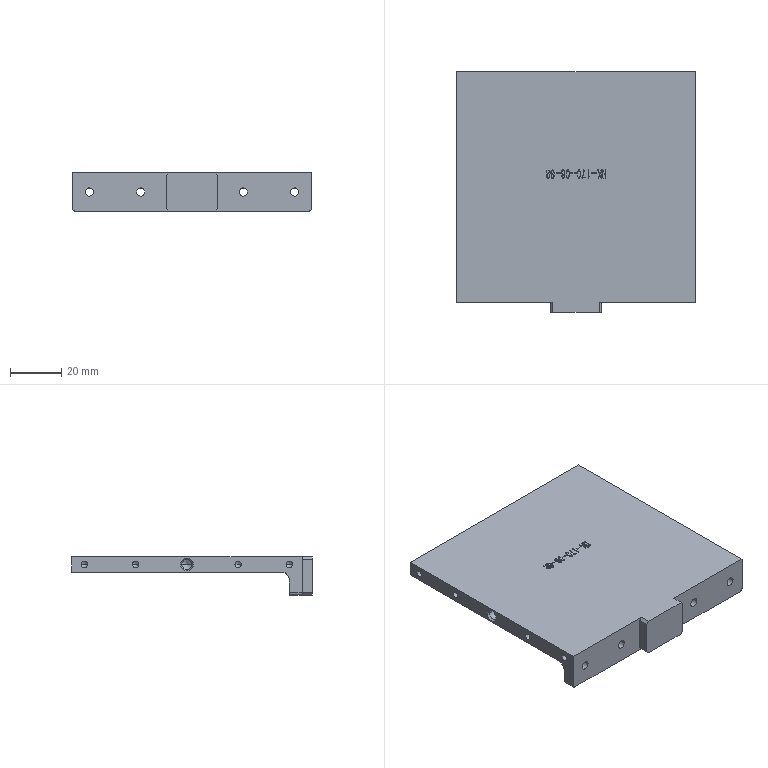NC program | NX | posted with a generic post | part box 93.2 x 94 x 15 mm
Whole program, first 2058 of 2264 lines:
N10 G17 G21 G94 G90
(FLOOR_WALL , TOOL : D10)
N12 T15 M6
N14 G54
N16 G17 G0 G90 X51. Y54.6 B0. C0. S9500 M3
N18 G43 Z30. H15
N20 Z-5.9
N22 G94 G1 Z-8.9 F1000.
N24 Y51.6
N26 Y-51.6 F3000.
N28 X50.005
N30 Y51.6
N32 X49.009
N34 Y-51.6
N36 X48.014
N38 Y51.6
N40 X47.019
N42 Y-51.6
N44 X46.023
N46 Y51.6
N48 X45.028
N50 Y-51.6
N52 X44.033
N54 Y51.6
N56 X43.037
N58 Y-51.6
N60 X42.042
N62 Y51.6
N64 X41.047
N66 Y-51.6
N68 X40.051
N70 Y51.6
N72 X39.056
N74 Y-51.6
N76 X38.061
N78 Y51.6
N80 X37.065
N82 Y-51.6
N84 X36.07
N86 Y51.6
N88 X35.075
N90 Y-51.6
N92 X34.079
N94 Y51.6
N96 X33.084
N98 Y-51.6
N100 X32.088
N102 Y51.6
N104 X31.093
N106 Y-51.6
N108 X30.098
N110 Y51.6
N112 X29.102
N114 Y-51.6
N116 X28.107
N118 Y51.6
N120 X27.112
N122 Y-51.6
N124 X26.116
N126 Y51.6
N128 X25.121
N130 Y-51.6
N132 X24.126
N134 Y51.6
N136 X23.13
N138 Y-51.6
N140 X22.135
N142 Y51.6
N144 X21.14
N146 Y-51.6
N148 X20.144
N150 Y51.6
N152 X19.149
N154 Y-51.6
N156 X18.154
N158 Y51.6
N160 X17.158
N162 Y-51.6
N164 X16.163
N166 Y51.6
N168 X15.168
N170 Y-51.6
N172 X14.172
N174 Y51.6
N176 X13.177
N178 Y-51.6
N180 X12.182
N182 Y51.6
N184 X11.186
N186 Y-51.6
N188 X10.191
N190 Y51.6
N192 X9.196
N194 Y-51.6
N196 X8.2
N198 Y51.6
N200 X7.205
N202 Y-51.6
N204 X6.21
N206 Y51.6
N208 X5.214
N210 Y-51.6
N212 X4.219
N214 Y51.6
N216 X3.224
N218 Y-51.6
N220 X2.228
N222 Y51.6
N224 X1.233
N226 Y-51.6
N228 X0.238
N230 Y51.6
N232 X-0.758
N234 Y-51.6
N236 X-1.753
N238 Y51.6
N240 X-2.749
N242 Y-51.6
N244 X-3.744
N246 Y51.6
N248 X-4.739
N250 Y-51.6
N252 X-5.735
N254 Y51.6
N256 X-6.73
N258 Y-51.6
N260 X-7.725
N262 Y51.6
N264 X-8.721
N266 Y-51.6
N268 X-9.716
N270 Y51.6
N272 X-10.711
N274 Y-51.6
N276 X-11.707
N278 Y51.6
N280 X-12.702
N282 Y-51.6
N284 X-13.697
N286 Y51.6
N288 X-14.693
N290 Y-51.6
N292 X-15.688
N294 Y51.6
N296 X-16.683
N298 Y-51.6
N300 X-17.679
N302 Y51.6
N304 X-18.674
N306 Y-51.6
N308 X-19.669
N310 Y51.6
N312 X-20.665
N314 Y-51.6
N316 X-21.66
N318 Y51.6
N320 X-22.655
N322 Y-51.6
N324 X-23.651
N326 Y51.6
N328 X-24.646
N330 Y-51.6
N332 X-25.641
N334 Y51.6
N336 X-26.637
N338 Y-51.6
N340 X-27.632
N342 Y51.6
N344 X-28.627
N346 Y-51.6
N348 X-29.623
N350 Y51.6
N352 X-30.618
N354 Y-51.6
N356 Y-54.75
N358 Z-5.9
N360 G0 Z30.
(FLOOR_WALL_1 , TOOL : D10)
N362 X2.833 Y6.4
N364 Z-7.5
N366 G1 X1.6 Z-7.565 F1000.
N368 Y-6.4 Z-8.235
N370 X14.4 Z-8.906
N372 Y6.4 Z-9.577
N374 X8. Z-9.913
N376 Y1.9
N378 X6.1 F3000.
N380 Y-1.9
N382 X9.9
N384 Y1.9
N386 X8.
N388 Y6.4
N390 X1.6
N392 Y-6.4
N394 X14.4
N396 Y6.4
N398 X8.
N400 Y13.4
N402 X-5.4
N404 Y-13.4
N406 X21.4
N408 Y13.4
N410 X8.
N412 Y20.4
N414 X-12.4
N416 Y-20.4
N418 X28.4
N420 Y20.4
N422 X8.
N424 Y27.4
N426 X-19.4
N428 Y-27.4
N430 X35.4
N432 Y27.4
N434 X8.
N436 Z-8.413
N438 G0 X2.833 Y6.4
N440 G1 X1.6 Z-8.477 F1000.
N442 Y-6.4 Z-9.148
N444 X14.4 Z-9.819
N446 Y6.4 Z-10.49
N448 X8. Z-10.825
N450 Y1.9
N452 X6.1 F3000.
N454 Y-1.9
N456 X9.9
N458 Y1.9
N460 X8.
N462 Y6.4
N464 X1.6
N466 Y-6.4
N468 X14.4
N470 Y6.4
N472 X8.
N474 Y13.4
N476 X-5.4
N478 Y-13.4
N480 X21.4
N482 Y13.4
N484 X8.
N486 Y20.4
N488 X-12.4
N490 Y-20.4
N492 X28.4
N494 Y20.4
N496 X8.
N498 Y27.4
N500 X-19.4
N502 Y-27.4
N504 X35.4
N506 Y27.4
N508 X8.
N510 Z-9.325
N512 G0 X2.833 Y6.4
N514 G1 X1.6 Z-9.39 F1000.
N516 Y-6.4 Z-10.06
N518 X14.4 Z-10.731
N520 Y6.4 Z-11.402
N522 X8. Z-11.738
N524 Y1.9
N526 X6.1 F3000.
N528 Y-1.9
N530 X9.9
N532 Y1.9
N534 X8.
N536 Y6.4
N538 X1.6
N540 Y-6.4
N542 X14.4
N544 Y6.4
N546 X8.
N548 Y13.4
N550 X-5.4
N552 Y-13.4
N554 X21.4
N556 Y13.4
N558 X8.
N560 Y20.4
N562 X-12.4
N564 Y-20.4
N566 X28.4
N568 Y20.4
N570 X8.
N572 Y27.4
N574 X-19.4
N576 Y-27.4
N578 X35.4
N580 Y27.4
N582 X8.
N584 Z-10.238
N586 G0 X2.833 Y6.4
N588 G1 X1.6 Z-10.302 F1000.
N590 Y-6.4 Z-10.973
N592 X14.4 Z-11.644
N594 Y6.4 Z-12.315
N596 X8. Z-12.65
N598 Y1.9
N600 X6.1 F3000.
N602 Y-1.9
N604 X9.9
N606 Y1.9
N608 X8.
N610 Y6.4
N612 X1.6
N614 Y-6.4
N616 X14.4
N618 Y6.4
N620 X8.
N622 Y13.4
N624 X-5.4
N626 Y-13.4
N628 X21.4
N630 Y13.4
N632 X8.
N634 Y20.4
N636 X-12.4
N638 Y-20.4
N640 X28.4
N642 Y20.4
N644 X8.
N646 Y27.4
N648 X-19.4
N650 Y-27.4
N652 X35.4
N654 Y27.4
N656 X8.
N658 Z-11.15
N660 G0 Z30.
N662 M5
(FLOOR_WALL_COPY , TOOL : D10JING)
N664 T14 M6
N666 G54
N668 G17 G0 G90 X52.975 Y52.74 B0. C0. S9500 M3
N670 G43 Z30. H14
N672 Z-8.
N674 G94 G1 Z-9. F1000.
N676 X52.5 Y52.466
N678 G3 X52. Y51.6 R1.
N680 G1 Y-51.6 F1500.
N682 X47.206
N684 Y51.6
N686 X42.412
N688 Y-51.6
N690 X37.618
N692 Y51.6
N694 X32.824
N696 Y-51.6
N698 X28.029
N700 Y51.6
N702 X23.235
N704 Y-51.6
N706 X18.441
N708 Y51.6
N710 X13.647
N712 Y-51.6
N714 X8.853
N716 Y51.6
N718 X4.059
N720 Y-51.6
N722 X-0.735
N724 Y51.6
N726 X-5.529
N728 Y-51.6
N730 X-10.324
N732 Y51.6
N734 X-15.118
N736 Y-51.6
N738 X-19.912
N740 Y51.6
N742 X-24.706
N744 Y-51.6
N746 X-29.5
N748 Y51.6
N750 G2 X-29. Y52.466 R1.
N752 G1 X-27.902 Y53.1
N754 Z-8.
N756 G0 Z30.
N758 X-28.402
N760 Z-8.
N762 G1 Z-9. F1000.
N764 X-29.5 Y52.466
N766 G3 X-30. Y51.6 R1.
N768 G1 Y-51.6 F1500.
N770 G3 X-29.5 Y-52.466 R1.
N772 G1 X-28.402 Y-53.1
N774 Z-8.
N776 G0 Z30.
N778 X-18.134 Y26.499
N780 Z-11.75
N782 G1 Z-12.75 F1000.
N784 G3 X-19. Y26.999 R1.
N786 G1 X35. F1500.
N788 Y22.09
N790 X-19.
N792 Y17.181
N794 X35.
N796 Y12.272
N798 X-19.
N800 Y7.363
N802 X35.
N804 Y2.454
N806 X-19.
N808 Y-2.455
N810 X35.
N812 Y-7.364
N814 X-19.
N816 Y-12.273
N818 X35.
N820 Y-17.182
N822 X-19.
N824 Y-22.091
N826 X35.
N828 Y-27.
N830 X-19.
N832 Y-26.134
N834 G3 X-19.5 Y-27. R1. F1000.
N836 G1 Y-27.5 F1500.
N838 X35.5
N840 Y27.5
N842 X-19.5
N844 Y-27.
N846 G3 X-19.25 Y-27.433 R0.5
N848 G1 X-18. Y-26.
N850 Z-11.75
N852 G0 Z30.
N854 M5
(ZLEVEL_PROFILE , TOOL : D4R0.5)
N856 T16 M6
N858 G54
N860 G17 G0 G90 X-35.319 Y49.295 B0. C0. S9500 M3
N862 G43 Z30. H16
N864 Z1.4
N866 G94 G1 Z-0.1 F1000.
N868 X-35.84 Y48.925
N870 G3 X-36.007 Y48.562 R0.4
N872 G1 X-36. Y48.49 F3000.
N874 Y46.087
N876 Y-46.567
N878 Y-48.49
N880 X-36.007 Y-48.562
N882 X-36.009 Y-48.603 Z-0.2
N884 X-36. Y-48.49
N886 Y-46.567
N888 Y46.087
N890 Y48.49
N892 X-36.009 Y48.603
N894 Y48.645 Z-0.3
N896 X-36. Y48.49
N898 Y46.087
N900 Y-46.567
N902 Y-48.49
N904 X-36.009 Y-48.645
N906 Y-48.687 Z-0.4
N908 X-36. Y-48.49
N910 Y-46.567
N912 Y46.087
N914 Y46.794
N916 Y48.49
N918 X-36.009 Y48.687
N920 X-36.006 Y48.728 Z-0.5
N922 X-36. Y48.49
N924 Y46.087
N926 Y-46.567
N928 Y-48.49
N930 X-36.006 Y-48.728
N932 X-36.002 Y-48.77 Z-0.6
N934 X-36. Y-48.49
N936 Y-46.567
N938 Y46.087
N940 X-36.002 Y48.77
N942 Y48.773 Z-0.7
N944 X-36. Y46.201
N946 Y-46.567
N948 Y-48.49
N950 X-36.002 Y-48.773
N952 Z-0.8
N954 X-36. Y-48.49
N956 Y-46.567
N958 Y46.314
N960 X-36.002 Y48.773
N962 Y48.774 Z-0.9
N964 X-36. Y46.228
N966 Y-46.567
N968 Y-48.49
N970 X-36.002 Y-48.774
N972 Z-1.
N974 X-36. Y-48.49
N976 Y-46.567
N978 Y46.228
N980 X-36.002 Y48.774
N982 Y48.775 Z-1.1
N984 X-36. Y46.228
N986 Y-46.567
N988 Y-48.49
N990 X-36.002 Y-48.775
N992 Z-1.2
N994 X-36. Y-48.49
N996 Y-46.567
N998 Y46.228
N1000 X-36.002 Y48.775
N1002 Z-1.3
N1004 X-36. Y46.228
N1006 Y-46.581
N1008 Y-48.49
N1010 X-36.002 Y-48.775
N1012 Y-48.776 Z-1.4
N1014 X-36. Y-48.49
N1016 Y-46.595
N1018 Y46.228
N1020 X-36.002 Y48.776
N1022 Z-1.5
N1024 X-36. Y46.228
N1026 Y-46.6
N1028 Y-48.49
N1030 X-36.002 Y-48.776
N1032 Y-48.777 Z-1.6
N1034 X-36. Y-48.49
N1036 Y-46.9
N1038 X-36.02 Y-46.879
N1040 G3 X-36. Y-46.612 R2.
N1042 G1 Y-46.578
N1044 Y46.228
N1046 X-36.002 Y48.777
N1048 Z-1.7
N1050 X-36. Y46.228
N1052 Y-46.578
N1054 Y-46.612
N1056 G2 X-36.02 Y-46.879 R2.
N1058 G1 X-36. Y-46.9
N1060 Y-48.49
N1062 X-36.002 Y-48.777
N1064 Z-1.8
N1066 X-36. Y-48.49
N1068 Y-46.9
N1070 X-36.02 Y-46.879
N1072 G3 X-36. Y-46.612 R2.
N1074 G1 Y-46.578
N1076 Y46.228
N1078 X-36.002 Y48.777
N1080 Y48.778 Z-1.9
N1082 X-36. Y46.228
N1084 Y-46.578
N1086 Y-46.612
N1088 G2 X-36.02 Y-46.879 R2.
N1090 G1 X-36. Y-46.9
N1092 Y-48.49
N1094 X-36.002 Y-48.778
N1096 Z-2.
N1098 X-36. Y-48.49
N1100 Y-46.9
N1102 X-36.02 Y-46.879
N1104 G3 X-36. Y-46.612 R2.
N1106 G1 Y-46.578
N1108 Y46.228
N1110 X-36.002 Y48.778
N1112 Z-2.1
N1114 X-36. Y46.228
N1116 Y-46.578
N1118 Y-46.612
N1120 G2 X-36.02 Y-46.879 R2.
N1122 G1 X-36. Y-46.9
N1124 Y-48.49
N1126 X-36.002 Y-48.778
N1128 Y-48.779 Z-2.2
N1130 X-36. Y-48.49
N1132 Y-46.9
N1134 X-36.02 Y-46.879
N1136 G3 X-36. Y-46.612 R2.
N1138 G1 Y-46.578
N1140 Y46.228
N1142 X-36.002 Y48.779
N1144 Z-2.3
N1146 X-36. Y46.228
N1148 Y-46.6
N1150 G2 X-36.02 Y-46.879 R2.
N1152 G1 X-36. Y-46.9
N1154 Y-48.49
N1156 X-36.002 Y-48.779
N1158 Y-48.78 Z-2.4
N1160 X-36. Y-48.49
N1162 Y-46.9
N1164 X-36.02 Y-46.879
N1166 G3 X-36. Y-46.6 R2.
N1168 G1 Y46.228
N1170 X-36.002 Y48.78
N1172 Z-2.5
N1174 X-36. Y46.228
N1176 Y-46.6
N1178 G2 X-36.02 Y-46.879 R2.
N1180 G1 X-36. Y-46.9
N1182 Y-48.49
N1184 X-36.002 Y-48.78
N1186 Z-2.6
N1188 X-36. Y-48.49
N1190 Y-46.9
N1192 X-36.02 Y-46.879
N1194 G3 X-36. Y-46.6 R2.
N1196 G1 Y46.228
N1198 X-36.002 Y48.78
N1200 Y48.781 Z-2.7
N1202 X-36. Y46.228
N1204 Y-46.6
N1206 G2 X-36.02 Y-46.879 R2.
N1208 G1 X-36. Y-46.9
N1210 Y-48.49
N1212 X-36.002 Y-48.781
N1214 Z-2.8
N1216 X-36. Y-48.49
N1218 Y-46.9
N1220 X-36.02 Y-46.879
N1222 G3 X-36. Y-46.6 R2.
N1224 G1 Y46.228
N1226 X-36.002 Y48.781
N1228 Y48.782 Z-2.9
N1230 X-36. Y46.228
N1232 Y-46.6
N1234 G2 X-36.02 Y-46.879 R2.
N1236 G1 X-36. Y-46.9
N1238 Y-48.49
N1240 X-36.002 Y-48.781
N1242 Y-48.782 Z-3.
N1244 X-36. Y-48.49
N1246 Y-46.9
N1248 X-36.02 Y-46.879
N1250 G3 X-36. Y-46.6 R2.
N1252 G1 Y46.228
N1254 X-36.002 Y48.782
N1256 Z-3.1
N1258 X-36. Y46.228
N1260 Y-46.6
N1262 G2 X-36.02 Y-46.879 R2.
N1264 G1 X-36. Y-46.9
N1266 Y-48.49
N1268 X-36.002 Y-48.782
N1270 Y-48.783 Z-3.2
N1272 X-36. Y-48.49
N1274 Y-46.9
N1276 X-36.02 Y-46.879
N1278 G3 X-36. Y-46.6 R2.
N1280 G1 Y46.228
N1282 X-36.002 Y48.783
N1284 Z-3.3
N1286 X-36. Y46.228
N1288 Y-46.6
N1290 G2 X-36.02 Y-46.879 R2.
N1292 G1 X-36. Y-46.9
N1294 Y-48.49
N1296 X-36.002 Y-48.783
N1298 Z-3.4
N1300 X-36. Y-48.49
N1302 Y-46.9
N1304 X-36.02 Y-46.879
N1306 G3 X-36. Y-46.6 R2.
N1308 G1 Y46.228
N1310 X-36.002 Y48.783
N1312 Y48.784 Z-3.5
N1314 X-36. Y46.228
N1316 Y-46.6
N1318 G2 X-36.02 Y-46.879 R2.
N1320 G1 X-36. Y-46.9
N1322 Y-48.49
N1324 X-36.002 Y-48.784
N1326 Z-3.6
N1328 X-36. Y-48.49
N1330 Y-46.9
N1332 X-36.02 Y-46.879
N1334 G3 X-36. Y-46.6 R2.
N1336 G1 Y46.228
N1338 X-36.002 Y48.784
N1340 Y48.785 Z-3.7
N1342 X-36. Y46.228
N1344 Y-46.6
N1346 G2 X-36.02 Y-46.879 R2.
N1348 G1 X-36. Y-46.9
N1350 Y-48.49
N1352 X-36.002 Y-48.784
N1354 Y-48.785 Z-3.8
N1356 X-36. Y-48.49
N1358 Y-46.9
N1360 X-36.02 Y-46.879
N1362 G3 X-36. Y-46.6 R2.
N1364 G1 Y46.228
N1366 X-36.001 Y48.785
N1368 Z-3.9
N1370 X-36. Y46.228
N1372 Y-46.6
N1374 G2 X-36.02 Y-46.879 R2.
N1376 G1 X-36. Y-46.9
N1378 Y-48.49
N1380 X-36.002 Y-48.785
N1382 Y-48.786 Z-4.
N1384 X-36. Y-48.49
N1386 Y-46.9
N1388 X-36.02 Y-46.879
N1390 G3 X-36. Y-46.6 R2.
N1392 G1 Y46.228
N1394 X-36.001 Y48.786
N1396 Z-4.1
N1398 X-36. Y46.228
N1400 Y-46.6
N1402 G2 X-36.02 Y-46.879 R2.
N1404 G1 X-36. Y-46.9
N1406 X-36.002 Y-48.786
N1408 X-36.001 Z-4.2
N1410 X-36. Y-46.9
N1412 X-36.02 Y-46.879
N1414 G3 X-36. Y-46.6 R2.
N1416 G1 Y46.228
N1418 X-36.001 Y48.787
N1420 Z-4.3
N1422 X-36. Y46.228
N1424 Y-46.6
N1426 G2 X-36.02 Y-46.879 R2.
N1428 G1 X-36. Y-46.9
N1430 X-36.001 Y-48.787
N1432 Z-4.4
N1434 X-36. Y-46.9
N1436 X-36.02 Y-46.879
N1438 G3 X-36. Y-46.6 R2.
N1440 G1 Y46.228
N1442 X-36.001 Y48.787
N1444 Y48.788 Z-4.5
N1446 X-36. Y46.228
N1448 Y-46.6
N1450 G2 X-36.02 Y-46.879 R2.
N1452 G1 X-36. Y-46.9
N1454 X-36.001 Y-48.787
N1456 Y-48.788 Z-4.6
N1458 X-36. Y-46.9
N1460 X-36.02 Y-46.879
N1462 G3 X-36. Y-46.6 R2.
N1464 G1 Y46.228
N1466 X-36.001 Y48.788
N1468 Z-4.7
N1470 X-36. Y46.228
N1472 Y-46.6
N1474 G2 X-36.02 Y-46.879 R2.
N1476 G1 X-36. Y-46.9
N1478 X-36.001 Y-48.788
N1480 Y-48.789 Z-4.8
N1482 X-36. Y-46.9
N1484 X-36.02 Y-46.879
N1486 G3 X-36. Y-46.6 R2.
N1488 G1 Y46.228
N1490 X-36.001 Y48.789
N1492 Z-4.9
N1494 X-36. Y46.228
N1496 Y-46.6
N1498 G2 X-36.02 Y-46.879 R2.
N1500 G1 X-36. Y-46.9
N1502 X-36.001 Y-48.789
N1504 Z-5.
N1506 X-36. Y-46.9
N1508 X-36.02 Y-46.879
N1510 G3 X-36. Y-46.6 R2.
N1512 G1 Y46.228
N1514 X-36.001 Y48.79
N1516 Z-5.1
N1518 X-36. Y46.228
N1520 Y-46.6
N1522 G2 X-36.02 Y-46.879 R2.
N1524 G1 X-36. Y-46.9
N1526 X-36.001 Y-48.79
N1528 Z-5.2
N1530 X-36. Y-46.9
N1532 X-36.02 Y-46.879
N1534 G3 X-36. Y-46.6 R2.
N1536 G1 Y46.228
N1538 X-36.001 Y48.79
N1540 Y48.791 Z-5.3
N1542 X-36. Y46.228
N1544 Y-46.6
N1546 G2 X-36.02 Y-46.879 R2.
N1548 G1 X-36. Y-46.9
N1550 X-36.001 Y-48.791
N1552 Z-5.4
N1554 X-36. Y-46.9
N1556 X-36.02 Y-46.879
N1558 G3 X-36. Y-46.6 R2.
N1560 G1 Y46.228
N1562 X-36.001 Y48.791
N1564 Z-5.5
N1566 X-36. Y46.228
N1568 Y-46.6
N1570 G2 X-36.02 Y-46.879 R2.
N1572 G1 X-36. Y-46.9
N1574 X-36.001 Y-48.791
N1576 Y-48.792 Z-5.6
N1578 X-36. Y-48.773
N1580 Y-46.9
N1582 X-36.02 Y-46.879
N1584 G3 X-36. Y-46.6 R2.
N1586 G1 Y46.228
N1588 X-36.001 Y48.792
N1590 Z-5.7
N1592 X-36. Y46.228
N1594 Y-46.6
N1596 G2 X-36.02 Y-46.879 R2.
N1598 G1 X-36. Y-46.9
N1600 Y-48.773
N1602 X-36.001 Y-48.792
N1604 Z-5.8
N1606 X-36. Y-48.773
N1608 Y-46.9
N1610 X-36.02 Y-46.879
N1612 G3 X-36. Y-46.6 R2.
N1614 G1 Y46.228
N1616 X-36.001 Y48.793
N1618 Z-5.9
N1620 X-36. Y46.228
N1622 Y-46.6
N1624 G2 X-36.02 Y-46.879 R2.
N1626 G1 X-36. Y-46.9
N1628 Y-48.773
N1630 X-36.001 Y-48.793
N1632 Z-6.
N1634 X-36. Y-48.773
N1636 Y-46.9
N1638 X-36.02 Y-46.879
N1640 G3 X-36. Y-46.6 R2.
N1642 G1 Y46.228
N1644 X-36.001 Y48.793
N1646 Y48.794 Z-6.1
N1648 X-36. Y46.228
N1650 Y-46.6
N1652 G2 X-36.02 Y-46.879 R2.
N1654 G1 X-36. Y-46.9
N1656 Y-48.773
N1658 X-36.001 Y-48.794
N1660 Z-6.2
N1662 X-36. Y-48.773
N1664 Y-46.9
N1666 X-36.02 Y-46.879
N1668 G3 X-36. Y-46.6 R2.
N1670 G1 Y46.228
N1672 X-36.001 Y48.794
N1674 Z-6.3
N1676 X-36. Y46.228
N1678 Y-46.6
N1680 G2 X-36.02 Y-46.879 R2.
N1682 G1 X-36. Y-46.9
N1684 Y-48.773
N1686 X-36.001 Y-48.794
N1688 Y-48.795 Z-6.4
N1690 X-36. Y-48.773
N1692 Y-46.9
N1694 X-36.02 Y-46.879
N1696 G3 X-36. Y-46.6 R2.
N1698 G1 Y46.228
N1700 X-36.001 Y48.795
N1702 X-35.998 Z-6.5
N1704 X-36. Y46.228
N1706 Y40.687
N1708 X-35.997 Y40.573
N1710 X-36. Y39.313
N1712 Y-19.313
N1714 X-35.996 Y-20.499
N1716 X-36. Y-20.687
N1718 Y-39.313
N1720 X-35.998 Y-40.573
N1722 X-36. Y-40.687
N1724 X-35.999 Y-46.6
N1726 X-35.995 Y-48.773
N1728 X-35.996 Y-48.795
N1730 X-35.987 Y-48.796 Z-6.55
N1732 X-35.982 Y-48.797 Z-6.6
N1734 X-35.99 Y-46.697
N1736 X-35.998 Y-46.511
N1738 Y-40.902
N1740 X-35.992 Y-40.573
N1742 X-35.998 Y-39.098
N1744 Y-20.902
N1746 G3 X-35.998 Y-19.085 R48.582
N1748 G1 Y19.085
N1750 X-35.993 Y19.368
N1752 G3 X-35.998 Y20.902 R90.14
N1754 G1 Y39.098
N1756 X-35.992 Y39.442
N1758 X-35.998 Y40.902
N1760 Y46.6
N1762 G3 X-35.987 Y46.828 R2.579
N1764 G1 X-35.982 Y48.49
N1766 X-35.986 Y48.796
N1768 X-35.975 Y48.797 Z-6.65
N1770 X-35.973 Z-6.7
N1772 X-35.968 Y48.49
N1774 X-35.976 Y46.836
N1776 G2 X-35.992 Y46.6 R1.944
N1778 G1 Y41.065
N1780 X-35.986 Y40.856
N1782 Y39.16
N1784 X-35.992 Y38.935
N1786 Y21.065
N1788 X-35.985 Y20.781
N1790 X-35.992 Y18.935
N1792 Y-18.935
N1794 X-35.985 Y-20.781
N1796 X-35.992 Y-21.065
N1798 Y-38.935
N1800 X-35.986 Y-39.16
N1802 Y-40.856
N1804 X-35.992 Y-41.065
N1806 Y-46.511
N1808 G2 X-35.975 Y-46.997 R8.136
N1810 G1 X-35.966 Y-48.798
N1812 X-35.956 Y-48.799 Z-6.749
N1814 X-35.947 Z-6.799
N1816 X-35.957 Y-47.359
N1818 G3 X-35.982 Y-46.511 R12.941
N1820 G1 Y-41.191
N1822 X-35.979 Y-41.139
N1824 X-35.978 Y-38.877
N1826 X-35.982 Y-38.809
N1828 Y-21.191
N1830 X-35.975 Y-21.064
N1832 X-35.976 Y-19.085
N1834 X-35.982 Y-18.802
N1836 Y18.802
N1838 X-35.976 Y20.781
N1840 X-35.982 Y21.191
N1842 Y38.809
N1844 X-35.978 Y38.877
N1846 X-35.979 Y41.139
N1848 X-35.982 Y41.191
N1850 Y46.511
N1852 X-35.966 Y46.794
N1854 X-35.949 Y48.49
N1856 X-35.955 Y48.798
N1858 X-35.946 Y48.799 Z-6.849
N1860 X-35.934 Y48.8 Z-6.898
N1862 X-35.929 Y48.49
N1864 X-35.946 Y46.794
N1866 X-35.968 Y46.511
N1868 Y41.295
N1870 X-35.961 Y41.139
N1872 X-35.965 Y39.725
N1874 X-35.961 Y38.877
N1876 X-35.968 Y38.705
N1878 Y21.295
N1880 X-35.963 Y18.802
N1882 X-35.968 Y18.705
N1884 Y-18.705
N1886 X-35.964 Y-18.802
N1888 X-35.965 Y-20.781
N1890 X-35.959 Y-21.064
N1892 X-35.968 Y-21.295
N1894 Y-38.705
N1896 X-35.961 Y-38.877
N1898 X-35.965 Y-40.008
N1900 X-35.961 Y-41.139
N1902 X-35.968 Y-41.295
N1904 Y-46.511
N1906 G2 X-35.94 Y-47.047 R6.034
N1908 G1 X-35.926 Y-48.8
N1910 X-35.913 Y-48.799 Z-6.947
N1912 X-35.903 Z-6.996
N1914 X-35.912 Y-47.359
N1916 X-35.918 Y-47.076
N1918 G3 X-35.95 Y-46.44 R6.566
N1920 G1 Y-41.377
N1922 X-35.943 Y-41.139
N1924 X-35.944 Y-38.877
N1926 X-35.95 Y-38.623
N1928 Y-21.377
N1930 X-35.942 Y-21.064
N1932 X-35.945 Y-18.802
N1934 X-35.95 Y-18.623
N1936 Y18.623
N1938 X-35.945 Y18.802
N1940 Y21.064
N1942 X-35.95 Y21.377
N1944 Y38.594
N1946 X-35.943 Y38.877
N1948 X-35.944 Y41.139
N1950 X-35.95 Y41.377
N1952 Y46.44
N1954 X-35.923 Y46.794
N1956 X-35.918 Y47.076
N1958 X-35.904 Y48.49
N1960 X-35.909 Y48.799
N1962 X-35.895 Z-7.045
N1964 X-35.883 Z-7.094
N1966 X-35.88 Y48.49
N1968 X-35.892 Y47.076
N1970 X-35.898 Y46.794
N1972 G3 X-35.928 Y46.228 R6.946
N1974 G1 Y41.448
N1976 X-35.922 Y41.139
N1978 X-35.926 Y38.564
N1980 X-35.928 Y38.552
N1982 Y21.448
N1984 X-35.925 Y21.347
N1986 X-35.922 Y18.802
N1988 X-35.928 Y18.552
N1990 Y-18.55
N1992 X-35.923 Y-18.802
N1994 X-35.925 Y-21.347
N1996 X-35.928 Y-21.448
N1998 Y-38.552
N2000 X-35.926 Y-38.564
N2002 X-35.921 Y-41.139
N2004 X-35.928 Y-41.448
N2006 Y-46.228
N2008 G3 X-35.898 Y-46.794 R5.294
N2010 G1 X-35.892 Y-47.076
N2012 X-35.879 Y-48.798
N2014 X-35.866 Z-7.142
N2016 X-35.853 Z-7.19
N2018 G3 X-35.873 Y-46.794 R59.222
N2020 G1 X-35.893 Y-46.511
N2022 X-35.903 Y-46.464
N2024 Y-41.507
N2026 X-35.898 Y-41.458
N2028 Y-38.543
N2030 X-35.903 Y-38.493
N2032 Y-21.507
N2034 X-35.896 Y-21.347
N2036 X-35.899 Y-18.508
N2038 X-35.903 Y-18.493
N2040 Y18.493
N2042 X-35.894 Y18.802
N2044 X-35.897 Y21.474
N2046 X-35.903 Y21.507
N2048 Y38.493
N2050 X-35.898 Y38.542
N2052 Y41.458
N2054 X-35.903 Y41.507
N2056 Y46.444
N2058 X-35.894 Y46.484
N2060 X-35.873 Y46.794
N2062 X-35.866 Y47.076
N2064 X-35.856 Y48.798
N2066 X-35.838 Z-7.238
N2068 X-35.823 Z-7.285
N2070 X-35.821 Y48.773
N2072 X-35.826 Y47.359
N2074 X-35.835 Y46.917
N2076 G2 X-35.873 Y46.465 R3.555
N2078 G1 Y41.552
N2080 X-35.868 Y41.139
N2082 X-35.869 Y38.594
N2084 X-35.873 Y38.448
N2086 Y21.552
N2088 X-35.869 Y21.508
N2090 Y18.519
N2092 X-35.873 Y18.448
N2094 Y-18.448
N2096 X-35.87 Y-18.49
N2098 X-35.869 Y-21.508
N2100 X-35.873 Y-21.552
N2102 Y-38.448
N2104 X-35.87 Y-38.594
N2106 X-35.867 Y-41.139
N2108 X-35.873 Y-41.552
N2110 Y-46.465
N2112 G2 X-35.836 Y-46.919 R3.835
N2114 G1 X-35.825 Y-47.359
N2116 X-35.82 Y-48.773
N2118 X-35.822 Y-48.798
N2120 X-35.808 Z-7.332
N2122 X-35.789 Z-7.379
N2124 X-35.788 Y-48.773
N2126 X-35.791 Y-47.359
N2128 X-35.8 Y-46.913
N2130 G3 X-35.84 Y-46.426 R4.088
N2132 G1 Y-41.588
N2134 X-35.834 Y-41.421
N2136 Y-38.594
N2138 X-35.84 Y-38.412
N2140 Y-21.588
N2142 X-35.833 Y-21.347
N2144 Y-18.802
N2146 X-35.84 Y-18.412
N2148 Y18.412
N2150 X-35.837 Y18.519
N2152 X-35.834 Y21.347
N2154 X-35.84 Y21.588
N2156 Y38.412
N2158 X-35.834 Y38.594
N2160 X-35.835 Y41.421
N2162 X-35.84 Y41.588
N2164 Y46.426
N2166 G3 X-35.8 Y46.912 R3.928
N2168 G1 X-35.791 Y47.359
N2170 X-35.788 Y48.773
N2172 X-35.79 Y48.798
N2174 X-35.769 Z-7.426
N2176 X-35.748 Y48.799 Z-7.472
N2178 G2 X-35.766 Y46.794 R38.008
N2180 G3 X-35.803 Y46.228 R4.94
N2182 G1 Y41.615
N2184 X-35.798 Y41.421
N2186 Y38.594
N2188 X-35.803 Y38.385
N2190 Y21.615
N2192 X-35.799 Y21.592
N2194 Y18.519
N2196 X-35.803 Y18.385
N2198 Y-18.385
N2200 X-35.8 Y-18.445
N2202 X-35.799 Y-21.592
N2204 X-35.803 Y-21.615
N2206 Y-38.385
N2208 X-35.798 Y-38.594
N2210 Y-41.421
N2212 X-35.803 Y-41.615
N2214 Y-46.228
N2216 G3 X-35.766 Y-46.794 R4.685
N2218 G2 X-35.748 Y-48.798 R44.761
N2220 G1 X-35.731 Z-7.517
N2222 X-35.707 Y-48.799 Z-7.563
N2224 X-35.705 Y-48.773
N2226 X-35.706 Y-47.496
N2228 G3 X-35.763 Y-46.449 R9.927
N2230 G1 Y-41.633
N2232 X-35.756 Y-41.567
N2234 X-35.758 Y-40.008
N2236 X-35.756 Y-38.433
N2238 X-35.763 Y-38.367
N2240 Y-21.633
N2242 X-35.753 Y-21.347
N2244 X-35.758 Y-19.933
N2246 X-35.755 Y-18.519
N2248 X-35.763 Y-18.367
N2250 Y18.367
N2252 X-35.756 Y18.519
N2254 X-35.758 Y20.216
N2256 X-35.754 Y20.499
N2258 G3 X-35.763 Y21.633 R20.866
N2260 G1 Y38.367
N2262 X-35.756 Y38.433
N2264 X-35.757 Y40.008
N2266 X-35.756 Y41.567
N2268 X-35.763 Y41.633
N2270 Y46.449
N2272 X-35.755 Y46.489
N2274 X-35.728 Y46.794
N2276 G3 X-35.707 Y48.799 R30.886
N2278 G1 X-35.693 Z-7.607
N2280 X-35.666 Y48.8 Z-7.652
N2282 X-35.664 Y48.773
N2284 X-35.666 Y47.172
N2286 G2 X-35.719 Y46.47 R4.697
N2288 G1 Y41.645
N2290 X-35.712 Y41.601
N2292 X-35.708 Y41.421
N2294 G3 X-35.709 Y38.594 R767.394
N2296 G1 X-35.712 Y38.399
N2298 X-35.719 Y38.355
N2300 Y21.645
N2302 X-35.708 Y21.347
N2304 X-35.716 Y19.933
N2306 G2 X-35.719 Y18.355 R28.843
N2308 G1 Y-18.355
N2310 X-35.712 Y-18.391
N2312 X-35.707 Y-18.802
N2314 G3 X-35.708 Y-21.347 R319.231
N2316 G1 X-35.715 Y-21.63
N2318 X-35.719 Y-21.645
N2320 Y-38.355
N2322 X-35.712 Y-38.399
N2324 X-35.708 Y-38.594
N2326 G3 X-35.709 Y-41.421 R797.189
N2328 G1 X-35.712 Y-41.601
N2330 X-35.719 Y-41.645
N2332 Y-46.47
N2334 G2 X-35.665 Y-47.177 R4.75
N2336 G1 X-35.664 Y-48.773
N2338 X-35.666 Y-48.8
N2340 X-35.642 Z-7.696
N2342 X-35.617 Z-7.739
N2344 X-35.623 Y-47.076
N2346 X-35.632 Y-46.794
N2348 G2 X-35.671 Y-46.228 R4.456
N2350 G1 Y-41.649
N2352 X-35.668 Y-41.635
N2354 Y-38.365
N2356 X-35.671 Y-38.351
N2358 Y-21.649
N2360 X-35.669 Y-21.63
N2362 X-35.668 Y-18.363
N2364 X-35.671 Y-18.351
N2366 Y18.351
N2368 X-35.666 Y18.519
N2370 X-35.669 Y21.63
N2372 X-35.671 Y21.649
N2374 Y38.351
N2376 X-35.668 Y38.365
N2378 Y41.635
N2380 X-35.671 Y41.649
N2382 Y46.228
N2384 G2 X-35.632 Y46.794 R4.483
N2386 G1 X-35.623 Y47.076
N2388 X-35.617 Y48.8
N2390 X-35.589 Z-7.782
N2392 X-35.565 Y48.799 Z-7.824
N2394 X-35.571 Y47.076
N2396 X-35.579 Y46.794
N2398 X-35.608 Y46.483
N2400 X-35.62 Y46.432
N2402 Y41.647
N2404 X-35.617 Y41.638
N2406 X-35.613 Y38.594
N2408 X-35.62 Y38.353
N2410 Y21.647
N2412 X-35.611 Y21.347
N2414 X-35.614 Y18.519
N2416 X-35.62 Y18.353
N2418 Y-18.353
N2420 X-35.617 Y-18.362
N2422 Y-21.63
N2424 X-35.62 Y-21.647
N2426 Y-38.353
N2428 X-35.617 Y-38.362
N2430 X-35.613 Y-41.421
N2432 X-35.62 Y-41.647
N2434 Y-46.432
N2436 X-35.608 Y-46.483
N2438 X-35.58 Y-46.794
N2440 X-35.571 Y-47.076
N2442 X-35.565 Y-48.799
N2444 X-35.538 Z-7.866
N2446 X-35.514 Z-7.907
N2448 X-35.52 Y-47.076
N2450 X-35.529 Y-46.794
N2452 X-35.556 Y-46.482
N2454 X-35.566 Y-46.461
N2456 Y-41.637
N2458 X-35.562 Y-41.624
N2460 Y-38.376
N2462 X-35.566 Y-38.363
N2464 Y-21.637
N2466 X-35.558 Y-21.347
N2468 X-35.562 Y-18.376
N2470 X-35.566 Y-18.363
N2472 Y18.363
N2474 X-35.562 Y18.376
N2476 X-35.556 Y21.347
N2478 X-35.566 Y21.637
N2480 Y38.363
N2482 X-35.562 Y38.376
N2484 Y41.624
N2486 X-35.566 Y41.637
N2488 Y46.45
N2490 X-35.556 Y46.482
N2492 X-35.529 Y46.794
N2494 X-35.52 Y47.076
N2496 X-35.514 Y48.799
N2498 X-35.479 Z-7.948
N2500 X-35.45 Z-7.988
N2502 X-35.448 Y48.773
N2504 X-35.449 Y47.359
N2506 X-35.465 Y46.824
N2508 G2 X-35.509 Y46.469 R1.953
N2510 G1 Y41.625
N2512 X-35.502 Y41.421
N2514 X-35.504 Y38.594
N2516 X-35.509 Y38.378
N2518 Y21.625
N2520 X-35.501 Y21.347
N2522 X-35.505 Y18.519
N2524 X-35.509 Y18.378
N2526 Y-18.375
N2528 X-35.5 Y-18.802
N2530 X-35.503 Y-21.347
N2532 X-35.509 Y-21.622
N2534 Y-38.375
N2536 X-35.502 Y-38.594
N2538 X-35.504 Y-41.421
N2540 X-35.509 Y-41.622
N2542 Y-46.469
N2544 G2 X-35.465 Y-46.824 R1.954
N2546 G1 X-35.449 Y-47.359
N2548 X-35.448 Y-48.773
N2550 X-35.45 Y-48.799
N2552 X-35.419 Y-48.8 Z-8.027
N2554 X-35.387 Z-8.066
N2556 X-35.385 Y-48.773
N2558 X-35.386 Y-47.359
N2560 X-35.4 Y-46.855
N2562 G3 X-35.449 Y-46.425 R2.549
N2564 G1 Y-41.602
N2566 X-35.444 Y-41.593
N2568 Y-38.407
N2570 X-35.449 Y-38.395
N2572 Y-21.602
N2574 X-35.439 Y-21.347
N2576 X-35.444 Y-18.407
N2578 X-35.449 Y-18.395
N2580 Y18.398
N2582 X-35.442 Y18.519
N2584 X-35.438 Y21.347
N2586 X-35.449 Y21.605
N2588 Y38.398
N2590 X-35.444 Y38.407
N2592 Y41.593
N2594 X-35.449 Y41.605
N2596 Y46.425
N2598 G3 X-35.4 Y46.856 R2.55
N2600 G1 X-35.386 Y47.359
N2602 X-35.385 Y48.773
N2604 X-35.387 Y48.8
N2606 X-35.354 Z-8.104
N2608 X-35.322 Z-8.141
N2610 X-35.32 Y48.773
N2612 X-35.321 Y47.359
N2614 X-35.335 Y46.861
N2616 G2 X-35.386 Y46.411 R2.707
N2618 G1 Y41.581
N2620 X-35.379 Y41.421
N2622 X-35.378 Y38.594
N2624 X-35.386 Y38.311
N2626 Y21.581
N2628 X-35.377 Y21.347
N2630 X-35.376 Y18.802
N2632 X-35.386 Y18.237
N2634 Y-18.419
N2636 X-35.375 Y-18.802
N2638 X-35.377 Y-21.347
N2640 X-35.386 Y-21.63
N2642 Y-38.419
N2644 X-35.378 Y-38.594
N2646 X-35.379 Y-41.421
N2648 X-35.386 Y-41.704
N2650 Y-46.411
N2652 G2 X-35.335 Y-46.861 R2.706
N2654 G1 X-35.321 Y-47.359
N2656 X-35.32 Y-48.773
N2658 X-35.322 Y-48.8
N2660 X-35.29 Z-8.178
N2662 X-35.258 Z-8.214
N2664 X-35.265 Y-47.076
N2666 X-35.273 Y-46.794
N2668 X-35.32 Y-46.433
N2670 Y-41.548
N2672 X-35.312 Y-41.421
N2674 X-35.311 Y-38.594
N2676 X-35.32 Y-38.448
N2678 Y-21.548
N2680 X-35.31 Y-21.347
N2682 X-35.311 Y-18.519
N2684 X-35.32 Y-18.448
N2686 Y18.237
N2688 X-35.311 Y18.519
N2690 X-35.31 Y21.347
N2692 X-35.32 Y21.552
N2694 Y38.452
N2696 X-35.312 Y38.594
N2698 Y41.421
N2700 X-35.32 Y41.552
N2702 Y46.433
N2704 X-35.273 Y46.794
N2706 X-35.265 Y47.076
N2708 X-35.258 Y48.8
N2710 X-35.22 Z-8.249
N2712 X-35.187 Z-8.284
N2714 X-35.195 Y47.076
N2716 X-35.206 Y46.794
N2718 X-35.251 Y46.43
N2720 Y41.52
N2722 X-35.246 Y41.421
N2724 Y38.594
N2726 X-35.251 Y38.484
N2728 Y21.52
N2730 X-35.245 Y21.347
N2732 X-35.244 Y18.488
N2734 X-35.251 Y18.237
N2736 Y-38.48
N2738 X-35.246 Y-38.594
N2740 Y-41.421
N2742 X-35.251 Y-41.516
N2744 Y-46.43
N2746 X-35.206 Y-46.794
N2748 X-35.195 Y-47.076
N2750 X-35.187 Y-48.8
N2752 X-35.146 Z-8.318
N2754 X-35.108 Y-48.801 Z-8.351
N2756 X-35.107 Y-48.773
N2758 X-35.108 Y-47.359
N2760 X-35.117 Y-47.076
N2762 X-35.159 Y-46.511
N2764 X-35.18 Y-46.405
N2766 Y-41.48
N2768 X-35.175 Y-41.421
N2770 X-35.168 Y-38.877
N2772 X-35.18 Y-38.517
N2774 Y-21.48
N2776 X-35.173 Y-21.347
N2778 X-35.169 Y-18.802
N2780 X-35.18 Y-18.517
N2782 Y18.237
N2784 X-35.169 Y18.802
N2786 X-35.173 Y21.347
N2788 X-35.18 Y21.483
N2790 Y38.52
N2792 X-35.175 Y38.594
N2794 X-35.168 Y41.139
N2796 X-35.18 Y41.483
N2798 Y46.405
N2800 X-35.174 Y46.416
N2802 X-35.128 Y46.794
N2804 X-35.117 Y47.076
N2806 X-35.108 Y48.801
N2808 X-35.069 Z-8.383
N2810 X-35.025 Z-8.415
N2812 X-35.023 Y48.773
N2814 X-35.024 Y47.359
N2816 X-35.035 Y47.076
N2818 X-35.087 Y46.495
N2820 X-35.107 Y46.402
N2822 Y41.444
N2824 X-35.103 Y41.421
N2826 X-35.107 Y38.311
N2828 Y21.444
N2830 X-35.094 Y21.064
N2832 X-35.097 Y18.802
N2834 X-35.107 Y18.519
N2836 Y-18.556
N2838 X-35.096 Y-18.802
N2840 X-35.101 Y-21.347
N2842 X-35.107 Y-21.63
N2844 Y-38.556
N2846 X-35.103 Y-38.594
N2848 X-35.107 Y-41.704
N2850 Y-46.402
N2852 X-35.087 Y-46.495
N2854 X-35.035 Y-47.076
N2856 X-35.024 Y-47.359
N2858 X-35.023 Y-48.773
N2860 X-35.025 Y-48.801
N2862 X-34.995 Z-8.445
N2864 X-34.942 Z-8.475
N2866 X-34.952 Y-47.076
N2868 X-34.965 Y-46.752
N2870 G3 X-35.032 Y-46.419 R1.067
N2872 G1 Y-41.399
N2874 X-35.02 Y-41.139
N2876 X-35.019 Y-38.877
N2878 X-35.032 Y-38.599
N2880 Y-21.63
N2882 X-35.026 Y-21.347
N2884 X-35.021 Y-18.802
N2886 X-35.032 Y-18.599
N2888 Y18.601
N2890 X-35.011 Y19.085
N2892 X-35.012 Y21.064
N2894 X-35.032 Y21.401
N2896 Y38.594
N2898 X-35.027 Y38.604
N2900 X-35.02 Y41.139
N2902 X-35.032 Y41.401
N2904 Y46.419
N2906 G3 X-34.966 Y46.742 R1.007
N2908 G1 X-34.952 Y47.076
N2910 X-34.942 Y48.801
N2912 X-34.944 Z-8.49
N2914 X-34.897 Y48.802 Z-8.518
N2916 X-34.864 Z-8.532
N2918 X-34.874 Y47.076
N2920 X-34.889 Y46.687
N2922 G2 X-34.956 Y46.418 R0.677
N2924 G1 Y41.357
N2926 G2 X-34.948 Y38.877 R36.976
N2928 G1 X-34.956 Y38.645
N2930 Y21.357
N2932 X-34.932 Y21.064
N2934 X-34.931 Y19.085
N2936 X-34.956 Y18.645
N2938 Y-18.643
N2940 X-34.931 Y-19.085
N2942 X-34.933 Y-21.064
N2944 X-34.956 Y-21.355
N2946 Y-38.643
N2948 X-34.947 Y-38.877
N2950 G2 X-34.956 Y-41.355 R36.047
N2952 G1 Y-46.418
N2954 G2 X-34.886 Y-46.717 R0.714
N2956 G1 X-34.863 Y-48.49
N2958 X-34.864 Y-48.802
N2960 X-34.83 Z-8.559
N2962 X-34.786 Z-8.586
N2964 X-34.81 Y-46.794
N2966 X-34.877 Y-46.358
N2968 Y-41.309
N2970 X-34.866 Y-41.139
N2972 X-34.865 Y-38.877
N2974 X-34.877 Y-38.691
N2976 Y-21.309
N2978 X-34.858 Y-21.064
N2980 X-34.855 Y-19.085
N2982 X-34.877 Y-18.691
N2984 Y18.691
N2986 X-34.856 Y19.085
N2988 X-34.858 Y21.064
N2990 X-34.877 Y21.309
N2992 Y38.691
N2994 X-34.865 Y38.877
N2996 X-34.866 Y41.139
N2998 X-34.877 Y41.309
N3000 Y46.348
N3002 X-34.81 Y46.794
N3004 X-34.786 Y48.802
N3006 X-34.745 Z-8.612
N3008 X-34.694 Y48.803 Z-8.637
N3010 X-34.692 Y48.773
N3012 X-34.72 Y46.794
N3014 X-34.798 Y46.339
N3016 Y41.261
N3018 X-34.787 Y41.139
N3020 X-34.786 Y38.877
N3022 X-34.798 Y38.739
N3024 Y21.261
N3026 X-34.777 Y20.781
N3028 X-34.79 Y18.802
N3030 X-34.798 Y18.739
N3032 Y-18.739
N3034 X-34.779 Y-19.085
N3036 X-34.783 Y-21.064
N3038 X-34.798 Y-21.261
N3040 Y-38.739
N3042 X-34.786 Y-38.877
N3044 X-34.787 Y-41.139
N3046 X-34.798 Y-41.261
N3048 Y-46.338
N3050 X-34.757 Y-46.511
N3052 X-34.694 Y-47.359
N3054 Y-48.803
N3056 X-34.666 Z-8.66
N3058 X-34.608 Z-8.684
N3060 X-34.609 Y-47.359
N3062 X-34.667 Y-46.511
N3064 X-34.717 Y-46.362
N3066 Y-41.211
N3068 X-34.692 Y-40.856
N3070 X-34.691 Y-39.16
N3072 X-34.717 Y-38.79
N3074 Y-21.211
N3076 X-34.697 Y-21.064
N3078 X-34.692 Y-19.085
N3080 X-34.717 Y-18.79
N3082 Y18.789
N3084 X-34.693 Y19.085
N3086 X-34.697 Y21.064
N3088 X-34.717 Y21.21
N3090 Y38.789
N3092 X-34.703 Y38.877
N3094 X-34.705 Y41.139
N3096 X-34.717 Y41.21
N3098 Y46.363
N3100 G3 X-34.633 Y46.794 R1.331
N3102 G1 X-34.608 Y48.803
N3104 X-34.581 Z-8.705
N3106 X-34.529 Y48.804 Z-8.727
N3108 X-34.553 Y46.794
N3110 G2 X-34.637 Y46.358 R1.177
N3112 G1 Y41.421
N3114 X-34.63 Y41.156
N3116 X-34.611 Y39.16
N3118 X-34.637 Y38.839
N3120 Y21.347
N3122 X-34.618 Y21.064
N3124 X-34.613 Y19.085
N3126 X-34.637 Y18.839
N3128 Y-18.802
N3130 X-34.613 Y-19.085
N3132 X-34.618 Y-21.064
N3134 X-34.637 Y-21.161
N3136 Y-38.594
N3138 X-34.628 Y-38.846
N3140 X-34.63 Y-41.139
N3142 X-34.637 Y-41.161
N3144 Y-46.369
N3146 X-34.613 Y-46.448
N3148 X-34.553 Y-46.794
N3150 X-34.529 Y-48.804
N3152 X-34.481 Z-8.747
N3154 X-34.433 Y-48.805 Z-8.766
N3156 X-34.465 Y-46.794
N3158 X-34.555 Y-46.326
N3160 Y-41.111
N3162 X-34.538 Y-40.856
N3164 X-34.537 Y-39.16
N3166 X-34.555 Y-38.877
N3168 Y-21.111
N3170 X-34.546 Y-21.064
N3172 X-34.539 Y-19.085
N3174 X-34.555 Y-18.802
N3176 Y18.889
N3178 X-34.54 Y19.085
N3180 X-34.546 Y21.064
N3182 X-34.555 Y21.347
N3184 Y38.889
N3186 X-34.538 Y39.16
N3188 Y40.856
N3190 X-34.555 Y41.139
N3192 Y46.307
N3194 X-34.466 Y46.794
N3196 X-34.433 Y48.81
N3198 X-34.39 Y48.813 Z-8.784
N3200 X-34.343 Y48.816 Z-8.802
N3202 X-34.377 Y46.794
N3204 X-34.433 Y46.412
N3206 X-34.475 Y46.296
N3208 Y41.139
N3210 X-34.451 Y40.856
N3212 X-34.452 Y39.16
N3214 X-34.475 Y38.938
N3216 Y21.064
N3218 X-34.449 Y20.781
N3220 X-34.455 Y19.085
N3222 X-34.475 Y18.938
N3224 Y-18.942
N3226 X-34.454 Y-19.085
N3228 X-34.45 Y-20.781
N3230 X-34.475 Y-21.062
N3232 Y-38.877
N3234 X-34.451 Y-39.16
N3236 X-34.452 Y-40.856
N3238 X-34.475 Y-41.062
N3240 Y-46.283
N3242 X-34.453 Y-46.369
N3244 X-34.364 Y-47.076
N3246 X-34.35 Y-47.359
N3248 X-34.341 Y-48.773
N3250 X-34.343 Y-48.806
N3252 X-34.308 Z-8.818
N3254 X-34.263 Y-48.807 Z-8.834
N3256 X-34.261 Y-48.773
N3258 X-34.272 Y-47.359
N3260 X-34.286 Y-47.076
N3262 X-34.346 Y-46.413
N3264 X-34.395 Y-46.276
N3266 Y-41.015
N3268 X-34.369 Y-40.856
N3270 X-34.368 Y-39.16
N3272 X-34.395 Y-38.877
N3274 Y-21.015
N3276 X-34.366 Y-20.781
N3278 X-34.371 Y-19.085
N3280 X-34.395 Y-18.989
N3282 Y18.985
N3284 X-34.372 Y19.085
N3286 X-34.365 Y20.781
N3288 X-34.395 Y21.064
N3290 Y38.877
N3292 X-34.377 Y38.995
N3294 X-34.368 Y40.856
N3296 X-34.395 Y41.139
N3298 Y46.286
N3300 X-34.35 Y46.402
N3302 X-34.297 Y46.794
N3304 X-34.262 Y48.822
N3306 X-34.216 Z-8.849
N3308 X-34.16 Z-8.863
N3310 X-34.239 Y46.676
N3312 X-34.317 Y46.3
N3314 Y41.139
N3316 X-34.295 Y40.856
N3318 X-34.302 Y39.039
N3320 X-34.317 Y38.877
N3322 Y21.064
N3324 X-34.292 Y20.781
N3326 X-34.299 Y19.085
N3328 X-34.317 Y19.031
N3330 Y-19.032
N3332 X-34.299 Y-19.085
N3334 X-34.293 Y-20.781
N3336 X-34.317 Y-20.969
N3338 Y-38.877
N3340 X-34.295 Y-39.16
N3342 X-34.296 Y-40.856
N3344 X-34.317 Y-41.139
N3346 Y-46.268
N3348 X-34.255 Y-46.511
N3350 X-34.165 Y-48.773
N3352 X-34.168 Y-48.808
N3354 X-34.118 Y-48.809 Z-8.875
N3356 X-34.074 Y-48.81 Z-8.887
N3358 X-34.071 Y-48.773
N3360 X-34.169 Y-46.511
N3362 X-34.243 Y-46.24
N3364 Y46.266
N3366 G3 X-34.059 Y48.822 R11.27
N3368 G1 X-34.014 Y48.821 Z-8.897
N3370 X-33.975 Z-8.907
N3372 X-34.051 Y46.794
N3374 X-34.136 Y46.345
N3376 X-34.174 Y46.239
N3378 Y40.891
N3380 X-34.161 Y40.856
N3382 X-34.158 Y39.16
N3384 X-34.174 Y39.109
N3386 Y20.891
N3388 X-34.143 Y20.781
N3390 X-34.136 Y19.368
N3392 X-34.174 Y19.109
N3394 Y-19.109
N3396 X-34.135 Y-19.368
N3398 X-34.145 Y-20.781
N3400 X-34.174 Y-20.891
N3402 Y-38.877
N3404 X-34.134 Y-40.573
N3406 X-34.174 Y-40.891
N3408 Y-46.2
N3410 X-34.091 Y-46.511
N3412 X-33.993 Y-48.773
N3414 X-33.997 Y-48.812
N3416 X-33.964 Y-48.81 Z-8.916
N3418 X-33.926 Y-48.808 Z-8.924
N3420 X-33.922 Y-48.773
N3422 X-34.025 Y-46.511
N3424 X-34.11 Y-46.187
N3426 Y-41.139
N3428 X-34.064 Y-39.442
N3430 X-34.11 Y-39.142
N3432 Y-20.857
N3434 X-34.078 Y-20.781
N3436 X-34.067 Y-19.368
N3438 X-34.11 Y-19.142
N3440 Y19.143
N3442 X-34.068 Y19.368
N3444 X-34.076 Y20.781
N3446 X-34.11 Y20.858
N3448 Y38.877
N3450 X-34.065 Y40.573
N3452 X-34.11 Y40.858
N3454 Y46.238
N3456 X-34.085 Y46.302
N3458 X-34.028 Y46.511
N3460 X-33.894 Y48.773
N3462 X-33.897 Y48.809
N3464 X-33.867 Y48.804 Z-8.932
N3466 X-33.827 Y48.796 Z-8.939
N3468 X-33.921 Y46.794
N3470 X-33.956 Y46.618
N3472 X-34.022 Y46.325
N3474 X-34.05 Y46.282
N3476 Y40.829
N3478 X-34.007 Y40.573
N3480 G2 X-34.05 Y39.16 R10.027
N3482 G1 Y20.829
N3484 G2 X-34.05 Y19.174 R6.128
N3486 G1 Y-19.171
N3488 X-34.009 Y-19.368
N3490 G2 X-34.05 Y-20.826 R9.992
N3492 G1 Y-39.171
N3494 X-34.006 Y-39.442
N3496 X-34.008 Y-40.573
N3498 X-34.05 Y-40.826
N3500 Y-45.945
N3502 X-34.041 Y-46.228
N3504 G2 X-33.968 Y-46.511 R51.916
N3506 G1 X-33.917 Y-46.794
N3508 X-33.84 Y-48.49
N3510 X-33.857 Y-48.797
N3512 X-33.847 Y-48.795 Z-8.945
N3514 X-33.801 Y-48.788 Z-8.951
N3516 X-33.783 Y-48.49
N3518 X-33.852 Y-46.794
N3520 X-33.957 Y-46.369
N3522 X-33.994 Y-46.306
N3524 Y-40.856
N3526 X-33.979 Y-40.798
N3528 X-33.958 Y-39.442
N3530 X-33.994 Y-39.195
N3532 Y-20.804
N3534 G3 X-33.961 Y-19.368 R11.24
N3536 G1 X-33.994 Y-19.195
N3538 Y19.196
N3540 G3 X-33.994 Y20.805 R6.692
N3542 G1 Y39.16
N3544 X-33.978 Y39.203
N3546 X-33.959 Y40.573
N3548 X-33.994 Y40.805
N3550 Y46.319
N3552 X-33.856 Y46.794
N3554 X-33.838 Y47.076
N3556 X-33.77 Y48.786
N3558 X-33.725 Y48.777 Z-8.96
N3560 X-33.789 Y47.076
N3562 X-33.805 Y46.794
N3564 X-33.944 Y46.351
N3566 Y40.785
N3568 X-33.891 Y40.573
N3570 Y39.442
N3572 X-33.944 Y39.202
N3574 Y20.785
N3576 G2 X-33.944 Y19.199 R4.048
N3578 G1 Y-19.215
N3580 X-33.895 Y-19.368
N3582 G2 X-33.944 Y-20.784 R6.704
N3584 G1 Y-39.215
N3586 X-33.89 Y-39.442
N3588 X-33.892 Y-40.573
N3590 X-33.944 Y-40.802
N3592 Y-46.346
N3594 X-33.801 Y-46.794
N3596 X-33.738 Y-48.49
N3598 X-33.757 Y-48.781
N3600 X-33.743 Y-48.779 Z-8.964
N3602 X-33.717 Y-48.775 Z-8.969
N3604 X-33.698 Y-48.49
N3606 X-33.755 Y-46.794
N3608 X-33.786 Y-46.511
N3610 X-33.894 Y-46.33
N3612 Y-40.76
N3614 X-33.829 Y-40.573
N3616 X-33.827 Y-39.442
N3618 X-33.894 Y-39.236
N3620 Y-20.76
N3622 X-33.825 Y-20.499
N3624 X-33.832 Y-19.368
N3626 X-33.894 Y-19.236
N3628 Y19.24
N3630 X-33.833 Y19.368
N3632 X-33.824 Y20.499
N3634 X-33.894 Y20.764
N3636 Y39.24
N3638 X-33.828 Y39.442
N3640 Y40.573
N3642 X-33.894 Y40.764
N3644 Y46.361
N3646 X-33.758 Y46.794
N3648 X-33.745 Y47.076
N3650 X-33.703 Y48.49
N3652 X-33.689 Y48.693
N3654 X-33.654 Y48.564 Z-8.976
N3656 X-33.672 Y48.413
N3658 X-33.691 Y47.359
N3660 X-33.705 Y47.076
N3662 X-33.716 Y46.794
N3664 X-33.843 Y46.369
N3666 Y40.747
N3668 X-33.772 Y40.573
N3670 X-33.771 Y39.442
N3672 X-33.843 Y39.256
N3674 Y20.747
N3676 G2 X-33.843 Y19.256 R3.075
N3678 G1 Y-19.253
N3680 G2 X-33.843 Y-20.744 R3.083
N3682 G1 Y-39.253
N3684 G2 X-33.769 Y-40.008 R1.52
N3686 X-33.843 Y-40.744 R1.425
N3688 G1 Y-46.329
N3690 X-33.737 Y-46.511
N3692 X-33.714 Y-46.794
N3694 X-33.654 Y-48.49
N3696 X-33.677 Y-48.762
N3698 X-33.607 Y-48.677 Z-8.982
N3700 X-33.668 Y-46.978
N3702 G3 X-33.796 Y-46.342 R1.993
N3704 G1 Y-40.73
N3706 X-33.726 Y-40.573
N3708 Y-39.442
N3710 X-33.796 Y-39.268
N3712 Y-20.73
N3714 G3 X-33.718 Y-20.216 R0.9
N3716 X-33.796 Y-19.268 R2.963
N3718 G1 Y19.27
N3720 G3 X-33.718 Y20.216 R2.919
N3722 X-33.796 Y20.732 R0.924
N3724 G1 Y39.27
N3726 X-33.725 Y39.442
N3728 G3 X-33.796 Y40.732 R4.018
N3730 G1 Y46.389
N3732 X-33.683 Y46.794
N3734 X-33.673 Y47.076
N3736 X-33.61 Y48.54
N3738 X-33.572 Y48.52 Z-8.987
N3740 G2 X-33.616 Y46.794 R11.109
N3742 G1 X-33.626 Y46.734
N3744 X-33.751 Y46.433
N3746 Y40.721
N3748 X-33.69 Y40.573
N3750 X-33.688 Y39.442
N3752 X-33.751 Y39.282
N3754 Y20.721
N3756 G2 X-33.751 Y19.282 R2.883
N3758 G1 Y-19.279
N3760 G2 X-33.751 Y-20.718 R2.811
N3762 G1 Y-39.279
N3764 X-33.689 Y-39.442
N3766 X-33.688 Y-40.573
N3768 X-33.751 Y-40.718
N3770 Y-46.34
N3772 G2 X-33.559 Y-48.601 R6.537
N3774 G1 X-33.514 Y-48.492 Z-8.994
N3776 X-33.45 Y-48.384 Z-9.
N3778 G2 X-33.612 Y-41.421 R162.78
N3780 G1 X-33.598 Y-41.35
N3782 X-33.386 Y-40.957
N3784 G3 X-33.6 Y-38.672 R2.065
N3786 G1 X-33.609 Y-21.347
N3788 G3 X-33.396 Y-19.099 R1.923
N3790 G1 X-33.571 Y-18.802
N3792 X-33.588 Y-18.74
N3794 X-33.602 Y-18.651
N3796 X-33.612 Y18.519
N3798 X-33.602 Y18.616
N3800 X-33.391 Y19.019
N3802 X-33.339 Y19.085
N3804 G3 X-33.596 Y21.277 R2.024
N3806 G1 X-33.598 Y38.665
N3808 G3 X-33.391 Y40.918 R1.667
N3810 G2 X-33.431 Y47.111 R17.284
N3812 X-33.453 Y48.366 R5.027
N3814 X-33.217 Y48.689 R0.4
N3816 G1 X-32.625 Y48.95
N3818 Z-7.5
N3820 G0 Z30.
(ZLEVEL_PROFILE_COPY , TOOL : D4R0.5)
N3822 X-45.87 Y47.893
N3824 Z1.488
N3826 G1 Z-0.012 F1000.
N3828 X-45.551 Y47.364
N3830 G3 X-45.2 Y47.17 R0.4
N3832 G1 X-43.281 Y47.207 F3000.
N3834 X-43. Y47.292
N3836 X-38.
N3838 G3 X-35.799 Y47.193 R11.499
N3840 G1 Y47.239 Z-0.019
N3842 Y47.27 Z-0.027
N3844 G2 X-38. Y47.381 R12.119
N3846 G1 X-43.
N3848 G2 X-45.2 Y47.26 R12.318
N3850 G1 Y47.323 Z-0.035
N3852 Y47.364 Z-0.043
N3854 G3 X-43. Y47.458 R9.462
N3856 G1 X-38.
N3858 G3 X-35.799 Y47.34 R15.599
N3860 G1 X-35.8 Y47.38 Z-0.054
N3862 Y47.406 Z-0.064
N3864 G2 X-38. Y47.534 R15.255
N3866 G1 X-43.
N3868 G2 X-45.2 Y47.432 R9.382
N3870 G1 X-45.199 Y47.474 Z-0.077
N3872 Y47.513 Z-0.09
N3874 G3 X-43. Y47.612 R8.605
N3876 G1 X-38.
N3878 G3 X-35.8 Y47.474 R18.275
N3880 G1 Y47.525 Z-0.106
N3882 Y47.557 Z-0.121
N3884 G2 X-38. Y47.691 R15.327
N3886 G1 X-43.
N3888 G2 X-45.2 Y47.584 R9.431
N3890 G1 Y47.628 Z-0.139
N3892 Y47.666 Z-0.158
N3894 G3 X-43. Y47.769 R11.28
N3896 G1 X-38.
N3898 G3 X-35.8 Y47.654 R13.527
N3900 G1 Y47.705 Z-0.179
N3902 Y47.755 Z-0.2
N3904 G2 X-38. Y47.849 R14.601
N3906 G1 X-43.
N3908 G2 X-45.2 Y47.758 R13.222
N3910 G1 Y47.804 Z-0.225
N3912 Y47.842 Z-0.249
N3914 G3 X-43. Y47.928 R13.918
N3916 G1 X-38.
N3918 G3 X-35.8 Y47.842 R12.199
N3920 G1 Y47.887 Z-0.277
N3922 Y47.925 Z-0.304
N3924 G2 X-38. Y48.005 R12.919
N3926 G1 X-43.
N3928 G2 X-45.2 Y47.925 R14.336
N3930 G1 Y47.965 Z-0.334
N3932 Y48.004 Z-0.364
N3934 G3 X-43. Y48.079 R15.083
N3936 G1 X-38.
N3938 G3 X-35.8 Y48.004 R13.763
N3940 G1 Y48.046 Z-0.397
N3942 Y48.087 Z-0.429
N3944 G2 X-38. Y48.151 R16.672
N3946 G1 X-43.
N3948 G2 X-45.2 Y48.087 R16.635
N3950 G1 Y48.122 Z-0.465
N3952 Y48.16 Z-0.5
N3954 G3 X-43. Y48.218 R17.947
N3956 G1 X-38.
N3958 G3 X-35.8 Y48.16 R17.465
N3960 G1 Y48.19 Z-0.538
N3962 Y48.22 Z-0.576
N3964 G2 X-38. Y48.281 R16.904
N3966 G1 X-43.
N3968 G2 X-45.2 Y48.22 R17.596
N3970 G1 Y48.251 Z-0.615
N3972 Y48.28 Z-0.655
N3974 G3 X-43. Y48.339 R17.833
N3976 G1 X-38.
N3978 G3 X-35.8 Y48.28 R17.359
N3980 G1 Y48.312 Z-0.697
N3982 Y48.343 Z-0.739
N3984 G2 X-38. Y48.392 R20.823
N3986 G1 X-43.
N3988 G2 X-45.2 Y48.343 R19.391
N3990 G1 Y48.37 Z-0.782
N3992 Y48.387 Z-0.826
N3994 X-44.95 Y48.388
N3996 X-43.837 Y48.389
N3998 G3 X-43. Y48.44 R23.568
N4000 G1 X-38.
N4002 G3 X-36.915 Y48.389 R11.588
N4004 G1 X-36.05 Y48.388
N4006 X-35.8 Y48.389
N4008 Y48.413 Z-0.871
N4010 Y48.432 Z-0.916
N4012 X-36.703 Y48.426
N4014 G2 X-38. Y48.482 R13.159
N4016 G1 X-43.
N4018 G2 X-43.838 Y48.436 R9.013
N4020 G1 X-45.2 Y48.426
N4022 Y48.449 Z-0.963
N4024 Y48.467 Z-1.009
N4026 X-44.95 Y48.471
N4028 X-43.837 Y48.475
N4030 X-43. Y48.518
N4032 X-38.
N4034 G3 X-35.8 Y48.476 R22.796
N4036 G1 X-35.911 Y48.513 Z-1.105
N4038 G2 X-38. Y48.547 R26.263
N4040 G1 X-43.
N4042 X-43.837 Y48.514
N4044 X-44.95 Y48.51
N4046 X-45.2 Y48.506
N4048 Y48.523 Z-1.153
N4050 Y48.54 Z-1.202
N4052 G3 X-43. Y48.57 R57.776
N4054 G1 X-38.
N4056 G3 X-35.911 Y48.546 R33.609
N4058 G1 Y48.551 Z-1.239
N4060 Y48.562 Z-1.277
N4062 G2 X-38. Y48.583 R41.177
N4064 G1 X-43.
N4066 G2 X-45.2 Y48.559 R56.051
N4068 G1 Y48.566 Z-1.314
N4070 Y48.576 Z-1.351
N4072 X-43.281 Y48.583
N4074 X-43. Y48.593
N4076 X-38.
N4078 X-37.719 Y48.585
N4080 X-36.05 Y48.577
N4082 X-35.911
N4084 Y48.585 Z-1.388
N4086 Y48.593 Z-1.426
N4088 X-45.2
N4090 X-45.199 Y48.598 Z-1.5
N4092 X-35.911 Y48.597
N4094 G3 X-35.565 Y48.797 R0.4
N4096 G1 X-35.248 Y49.345
N4098 Z0.
N4100 G0 Z30.
N4102 X-35.13 Y-47.893
N4104 Z1.488
N4106 G1 Z-0.012 F1000.
N4108 X-35.449 Y-47.364
N4110 G3 X-35.8 Y-47.17 R0.4
N4112 G1 X-37.719 Y-47.207 F3000.
N4114 X-38. Y-47.292